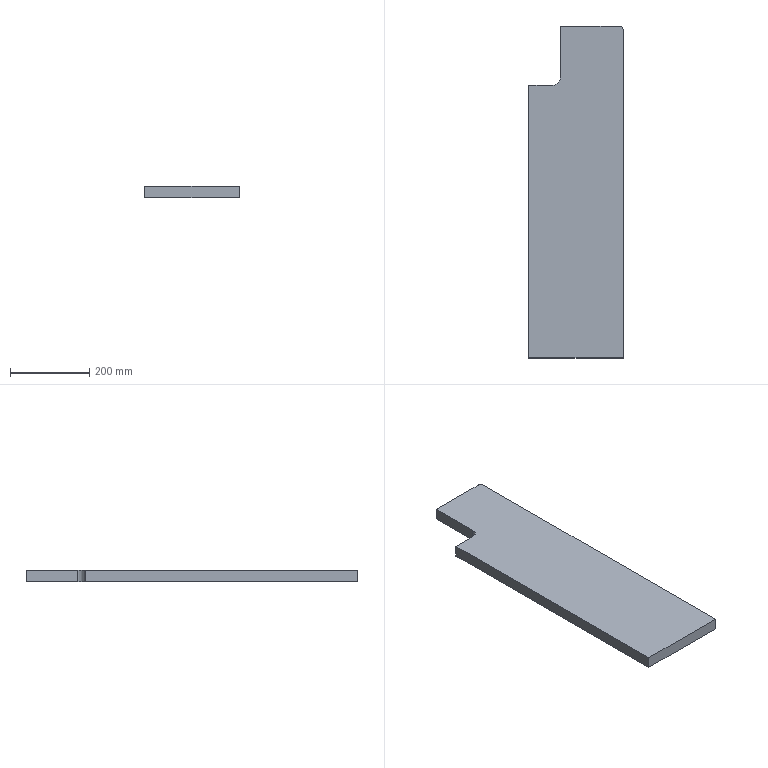Part | SolidWorks | features Extrusion 1, Fillet 1 | 1 solid | 10 faces | box 239 x 840 x 30 mm | volume 5664731 mm3 | plane 8 | cylinder 2 | commonest cylinder face diameters 20 x1 40 x1
STEP:
#1=CARTESIAN_POINT('',(0.,690.,0.));
#2=VERTEX_POINT('',#1);
#3=CARTESIAN_POINT('',(0.,0.,0.));
#4=VERTEX_POINT('',#3);
#5=CARTESIAN_POINT('',(0.,690.,0.));
#6=DIRECTION('',(0.,-1.,0.));
#7=VECTOR('',#6,1000.);
#8=LINE('',#5,#7);
#9=EDGE_CURVE('',#2,#4,#8,.T.);
#10=ORIENTED_EDGE('',*,*,#9,.T.);
#11=CARTESIAN_POINT('',(0.,0.,30.));
#12=VERTEX_POINT('',#11);
#13=CARTESIAN_POINT('',(0.,0.,30.));
#14=DIRECTION('',(0.,0.,-1.));
#15=VECTOR('',#14,1000.);
#16=LINE('',#13,#15);
#17=EDGE_CURVE('',#12,#4,#16,.T.);
#18=ORIENTED_EDGE('',*,*,#17,.F.);
#19=CARTESIAN_POINT('',(0.,690.,30.));
#20=VERTEX_POINT('',#19);
#21=CARTESIAN_POINT('',(0.,690.,30.));
#22=DIRECTION('',(0.,-1.,0.));
#23=VECTOR('',#22,1000.);
#24=LINE('',#21,#23);
#25=EDGE_CURVE('',#20,#12,#24,.T.);
#26=ORIENTED_EDGE('',*,*,#25,.F.);
#27=CARTESIAN_POINT('',(0.,690.,30.));
#28=DIRECTION('',(0.,0.,-1.));
#29=VECTOR('',#28,1000.);
#30=LINE('',#27,#29);
#31=EDGE_CURVE('',#20,#2,#30,.T.);
#32=ORIENTED_EDGE('',*,*,#31,.T.);
#33=EDGE_LOOP('',(#10,#18,#26,#32));
#34=FACE_OUTER_BOUND('',#33,.T.);
#35=CARTESIAN_POINT('',(0.,690.,30.));
#36=DIRECTION('',(1.,0.,0.));
#37=DIRECTION('',(0.,1.,0.));
#38=AXIS2_PLACEMENT_3D('',#35,#36,#37);
#39=PLANE('',#38);
#40=ADVANCED_FACE('',(#34),#39,.F.);
#41=CARTESIAN_POINT('',(239.,0.,0.));
#42=VERTEX_POINT('',#41);
#43=CARTESIAN_POINT('',(0.,0.,0.));
#44=DIRECTION('',(1.,0.,0.));
#45=VECTOR('',#44,1000.);
#46=LINE('',#43,#45);
#47=EDGE_CURVE('',#4,#42,#46,.T.);
#48=ORIENTED_EDGE('',*,*,#47,.T.);
#49=CARTESIAN_POINT('',(239.,0.,30.));
#50=VERTEX_POINT('',#49);
#51=CARTESIAN_POINT('',(239.,0.,30.));
#52=DIRECTION('',(0.,0.,-1.));
#53=VECTOR('',#52,1000.);
#54=LINE('',#51,#53);
#55=EDGE_CURVE('',#50,#42,#54,.T.);
#56=ORIENTED_EDGE('',*,*,#55,.F.);
#57=CARTESIAN_POINT('',(0.,0.,30.));
#58=DIRECTION('',(1.,0.,0.));
#59=VECTOR('',#58,1000.);
#60=LINE('',#57,#59);
#61=EDGE_CURVE('',#12,#50,#60,.T.);
#62=ORIENTED_EDGE('',*,*,#61,.F.);
#63=ORIENTED_EDGE('',*,*,#17,.T.);
#64=EDGE_LOOP('',(#48,#56,#62,#63));
#65=FACE_OUTER_BOUND('',#64,.T.);
#66=CARTESIAN_POINT('',(0.,0.,30.));
#67=DIRECTION('',(0.,1.,0.));
#68=DIRECTION('',(0.,0.,1.));
#69=AXIS2_PLACEMENT_3D('',#66,#67,#68);
#70=PLANE('',#69);
#71=ADVANCED_FACE('',(#65),#70,.F.);
#72=CARTESIAN_POINT('',(239.,830.,0.));
#73=VERTEX_POINT('',#72);
#74=CARTESIAN_POINT('',(239.,0.,0.));
#75=DIRECTION('',(0.,1.,0.));
#76=VECTOR('',#75,1000.);
#77=LINE('',#74,#76);
#78=EDGE_CURVE('',#42,#73,#77,.T.);
#79=ORIENTED_EDGE('',*,*,#78,.T.);
#80=CARTESIAN_POINT('',(239.,830.,30.));
#81=VERTEX_POINT('',#80);
#82=CARTESIAN_POINT('',(239.,830.,30.));
#83=DIRECTION('',(0.,0.,1.));
#84=VECTOR('',#83,1000.);
#85=LINE('',#82,#84);
#86=EDGE_CURVE('',#73,#81,#85,.T.);
#87=ORIENTED_EDGE('',*,*,#86,.T.);
#88=CARTESIAN_POINT('',(239.,0.,30.));
#89=DIRECTION('',(0.,1.,0.));
#90=VECTOR('',#89,1000.);
#91=LINE('',#88,#90);
#92=EDGE_CURVE('',#50,#81,#91,.T.);
#93=ORIENTED_EDGE('',*,*,#92,.F.);
#94=ORIENTED_EDGE('',*,*,#55,.T.);
#95=EDGE_LOOP('',(#79,#87,#93,#94));
#96=FACE_OUTER_BOUND('',#95,.T.);
#97=CARTESIAN_POINT('',(239.,0.,30.));
#98=DIRECTION('',(-1.,0.,0.));
#99=DIRECTION('',(0.,-1.,0.));
#100=AXIS2_PLACEMENT_3D('',#97,#98,#99);
#101=PLANE('',#100);
#102=ADVANCED_FACE('',(#96),#101,.F.);
#103=CARTESIAN_POINT('',(229.,840.,30.));
#104=VERTEX_POINT('',#103);
#105=CARTESIAN_POINT('',(80.,840.,30.));
#106=VERTEX_POINT('',#105);
#107=CARTESIAN_POINT('',(239.,840.,30.));
#108=DIRECTION('',(-1.,0.,0.));
#109=VECTOR('',#108,1000.);
#110=LINE('',#107,#109);
#111=EDGE_CURVE('',#104,#106,#110,.T.);
#112=ORIENTED_EDGE('',*,*,#111,.F.);
#113=CARTESIAN_POINT('',(229.,840.,0.));
#114=VERTEX_POINT('',#113);
#115=CARTESIAN_POINT('',(229.,840.,30.));
#116=DIRECTION('',(0.,0.,-1.));
#117=VECTOR('',#116,1000.);
#118=LINE('',#115,#117);
#119=EDGE_CURVE('',#104,#114,#118,.T.);
#120=ORIENTED_EDGE('',*,*,#119,.T.);
#121=CARTESIAN_POINT('',(80.,840.,0.));
#122=VERTEX_POINT('',#121);
#123=CARTESIAN_POINT('',(239.,840.,0.));
#124=DIRECTION('',(-1.,0.,0.));
#125=VECTOR('',#124,1000.);
#126=LINE('',#123,#125);
#127=EDGE_CURVE('',#114,#122,#126,.T.);
#128=ORIENTED_EDGE('',*,*,#127,.T.);
#129=CARTESIAN_POINT('',(80.,840.,30.));
#130=DIRECTION('',(0.,0.,-1.));
#131=VECTOR('',#130,1000.);
#132=LINE('',#129,#131);
#133=EDGE_CURVE('',#106,#122,#132,.T.);
#134=ORIENTED_EDGE('',*,*,#133,.F.);
#135=EDGE_LOOP('',(#112,#120,#128,#134));
#136=FACE_OUTER_BOUND('',#135,.T.);
#137=CARTESIAN_POINT('',(239.,840.,30.));
#138=DIRECTION('',(0.,-1.,0.));
#139=DIRECTION('',(0.,0.,-1.));
#140=AXIS2_PLACEMENT_3D('',#137,#138,#139);
#141=PLANE('',#140);
#142=ADVANCED_FACE('',(#136),#141,.F.);
#143=CARTESIAN_POINT('',(80.,710.,0.));
#144=VERTEX_POINT('',#143);
#145=CARTESIAN_POINT('',(80.,710.,0.));
#146=DIRECTION('',(0.,-1.,0.));
#147=VECTOR('',#146,1000.);
#148=LINE('',#145,#147);
#149=EDGE_CURVE('',#122,#144,#148,.T.);
#150=ORIENTED_EDGE('',*,*,#149,.T.);
#151=CARTESIAN_POINT('',(80.,710.,30.));
#152=VERTEX_POINT('',#151);
#153=CARTESIAN_POINT('',(80.,710.,30.));
#154=DIRECTION('',(0.,0.,-1.));
#155=VECTOR('',#154,1000.);
#156=LINE('',#153,#155);
#157=EDGE_CURVE('',#152,#144,#156,.T.);
#158=ORIENTED_EDGE('',*,*,#157,.F.);
#159=CARTESIAN_POINT('',(80.,710.,30.));
#160=DIRECTION('',(0.,-1.,0.));
#161=VECTOR('',#160,1000.);
#162=LINE('',#159,#161);
#163=EDGE_CURVE('',#106,#152,#162,.T.);
#164=ORIENTED_EDGE('',*,*,#163,.F.);
#165=ORIENTED_EDGE('',*,*,#133,.T.);
#166=EDGE_LOOP('',(#150,#158,#164,#165));
#167=FACE_OUTER_BOUND('',#166,.T.);
#168=CARTESIAN_POINT('',(80.,710.,30.));
#169=DIRECTION('',(1.,0.,0.));
#170=DIRECTION('',(0.,1.,0.));
#171=AXIS2_PLACEMENT_3D('',#168,#169,#170);
#172=PLANE('',#171);
#173=ADVANCED_FACE('',(#167),#172,.F.);
#174=CARTESIAN_POINT('',(60.,690.,0.));
#175=VERTEX_POINT('',#174);
#176=CARTESIAN_POINT('',(60.,710.,0.));
#177=DIRECTION('',(0.,0.,-1.));
#178=DIRECTION('',(1.,0.,0.));
#179=AXIS2_PLACEMENT_3D('',#176,#177,#178);
#180=CIRCLE('',#179,20.);
#181=EDGE_CURVE('',#144,#175,#180,.T.);
#182=ORIENTED_EDGE('',*,*,#181,.T.);
#183=CARTESIAN_POINT('',(60.,690.,30.));
#184=VERTEX_POINT('',#183);
#185=CARTESIAN_POINT('',(60.,690.,30.));
#186=DIRECTION('',(0.,0.,-1.));
#187=VECTOR('',#186,1000.);
#188=LINE('',#185,#187);
#189=EDGE_CURVE('',#184,#175,#188,.T.);
#190=ORIENTED_EDGE('',*,*,#189,.F.);
#191=CARTESIAN_POINT('',(60.,710.,30.));
#192=DIRECTION('',(0.,0.,-1.));
#193=DIRECTION('',(1.,0.,0.));
#194=AXIS2_PLACEMENT_3D('',#191,#192,#193);
#195=CIRCLE('',#194,20.);
#196=EDGE_CURVE('',#152,#184,#195,.T.);
#197=ORIENTED_EDGE('',*,*,#196,.F.);
#198=ORIENTED_EDGE('',*,*,#157,.T.);
#199=EDGE_LOOP('',(#182,#190,#197,#198));
#200=FACE_OUTER_BOUND('',#199,.T.);
#201=CARTESIAN_POINT('',(60.,710.,30.));
#202=DIRECTION('',(0.,0.,-1.));
#203=DIRECTION('',(-1.,0.,0.));
#204=AXIS2_PLACEMENT_3D('',#201,#202,#203);
#205=CYLINDRICAL_SURFACE('',#204,20.);
#206=ADVANCED_FACE('',(#200),#205,.F.);
#207=CARTESIAN_POINT('',(0.,690.,0.));
#208=DIRECTION('',(-1.,0.,0.));
#209=VECTOR('',#208,1000.);
#210=LINE('',#207,#209);
#211=EDGE_CURVE('',#175,#2,#210,.T.);
#212=ORIENTED_EDGE('',*,*,#211,.T.);
#213=ORIENTED_EDGE('',*,*,#31,.F.);
#214=CARTESIAN_POINT('',(0.,690.,30.));
#215=DIRECTION('',(-1.,0.,0.));
#216=VECTOR('',#215,1000.);
#217=LINE('',#214,#216);
#218=EDGE_CURVE('',#184,#20,#217,.T.);
#219=ORIENTED_EDGE('',*,*,#218,.F.);
#220=ORIENTED_EDGE('',*,*,#189,.T.);
#221=EDGE_LOOP('',(#212,#213,#219,#220));
#222=FACE_OUTER_BOUND('',#221,.T.);
#223=CARTESIAN_POINT('',(0.,690.,30.));
#224=DIRECTION('',(0.,-1.,0.));
#225=DIRECTION('',(0.,0.,-1.));
#226=AXIS2_PLACEMENT_3D('',#223,#224,#225);
#227=PLANE('',#226);
#228=ADVANCED_FACE('',(#222),#227,.F.);
#229=ORIENTED_EDGE('',*,*,#92,.T.);
#230=CARTESIAN_POINT('',(229.,830.,30.));
#231=DIRECTION('',(0.,0.,1.));
#232=DIRECTION('',(1.,0.,0.));
#233=AXIS2_PLACEMENT_3D('',#230,#231,#232);
#234=CIRCLE('',#233,10.);
#235=EDGE_CURVE('',#81,#104,#234,.T.);
#236=ORIENTED_EDGE('',*,*,#235,.T.);
#237=ORIENTED_EDGE('',*,*,#111,.T.);
#238=ORIENTED_EDGE('',*,*,#163,.T.);
#239=ORIENTED_EDGE('',*,*,#196,.T.);
#240=ORIENTED_EDGE('',*,*,#218,.T.);
#241=ORIENTED_EDGE('',*,*,#25,.T.);
#242=ORIENTED_EDGE('',*,*,#61,.T.);
#243=EDGE_LOOP('',(#229,#236,#237,#238,#239,#240,#241,#242));
#244=FACE_OUTER_BOUND('',#243,.T.);
#245=CARTESIAN_POINT('',(60.,710.,30.));
#246=DIRECTION('',(0.,0.,1.));
#247=DIRECTION('',(1.,0.,0.));
#248=AXIS2_PLACEMENT_3D('',#245,#246,#247);
#249=PLANE('',#248);
#250=ADVANCED_FACE('',(#244),#249,.T.);
#251=ORIENTED_EDGE('',*,*,#127,.F.);
#252=CARTESIAN_POINT('',(229.,830.,0.));
#253=DIRECTION('',(0.,0.,-1.));
#254=DIRECTION('',(1.,0.,0.));
#255=AXIS2_PLACEMENT_3D('',#252,#253,#254);
#256=CIRCLE('',#255,10.);
#257=EDGE_CURVE('',#114,#73,#256,.T.);
#258=ORIENTED_EDGE('',*,*,#257,.T.);
#259=ORIENTED_EDGE('',*,*,#78,.F.);
#260=ORIENTED_EDGE('',*,*,#47,.F.);
#261=ORIENTED_EDGE('',*,*,#9,.F.);
#262=ORIENTED_EDGE('',*,*,#211,.F.);
#263=ORIENTED_EDGE('',*,*,#181,.F.);
#264=ORIENTED_EDGE('',*,*,#149,.F.);
#265=EDGE_LOOP('',(#251,#258,#259,#260,#261,#262,#263,#264));
#266=FACE_OUTER_BOUND('',#265,.T.);
#267=CARTESIAN_POINT('',(60.,710.,0.));
#268=DIRECTION('',(0.,0.,1.));
#269=DIRECTION('',(1.,0.,0.));
#270=AXIS2_PLACEMENT_3D('',#267,#268,#269);
#271=PLANE('',#270);
#272=ADVANCED_FACE('',(#266),#271,.F.);
#273=ORIENTED_EDGE('',*,*,#235,.F.);
#274=ORIENTED_EDGE('',*,*,#86,.F.);
#275=ORIENTED_EDGE('',*,*,#257,.F.);
#276=ORIENTED_EDGE('',*,*,#119,.F.);
#277=EDGE_LOOP('',(#273,#274,#275,#276));
#278=FACE_OUTER_BOUND('',#277,.T.);
#279=CARTESIAN_POINT('',(229.,830.,30.));
#280=DIRECTION('',(0.,0.,-1.));
#281=DIRECTION('',(-1.,0.,0.));
#282=AXIS2_PLACEMENT_3D('',#279,#280,#281);
#283=CYLINDRICAL_SURFACE('',#282,10.);
#284=ADVANCED_FACE('',(#278),#283,.T.);
#285=CLOSED_SHELL('',(#40,#71,#102,#142,#173,#206,#228,#250,#272,#284));
#286=MANIFOLD_SOLID_BREP('',#285);
#287=CARTESIAN_POINT('',(0.,0.,0.));
#288=DIRECTION('',(0.,0.,1.));
#289=DIRECTION('',(1.,0.,0.));
#290=AXIS2_PLACEMENT_3D('',#287,#288,#289);
#291=(LENGTH_UNIT()NAMED_UNIT(*)SI_UNIT(.MILLI.,.METRE.));
#292=UNCERTAINTY_MEASURE_WITH_UNIT(LENGTH_MEASURE(0.00001),#291,'','');
#293=(NAMED_UNIT(*)PLANE_ANGLE_UNIT()SI_UNIT($,.RADIAN.));
#294=(NAMED_UNIT(*)SI_UNIT($,.STERADIAN.)SOLID_ANGLE_UNIT());
#295=(GEOMETRIC_REPRESENTATION_CONTEXT(3)GLOBAL_UNCERTAINTY_ASSIGNED_CONTEXT((#292))GLOBAL_UNIT_ASSIGNED_CONTEXT((#291,#293,#294))REPRESENTATION_CONTEXT('',''));
#296=ADVANCED_BREP_SHAPE_REPRESENTATION('',(#286,#290),#295);